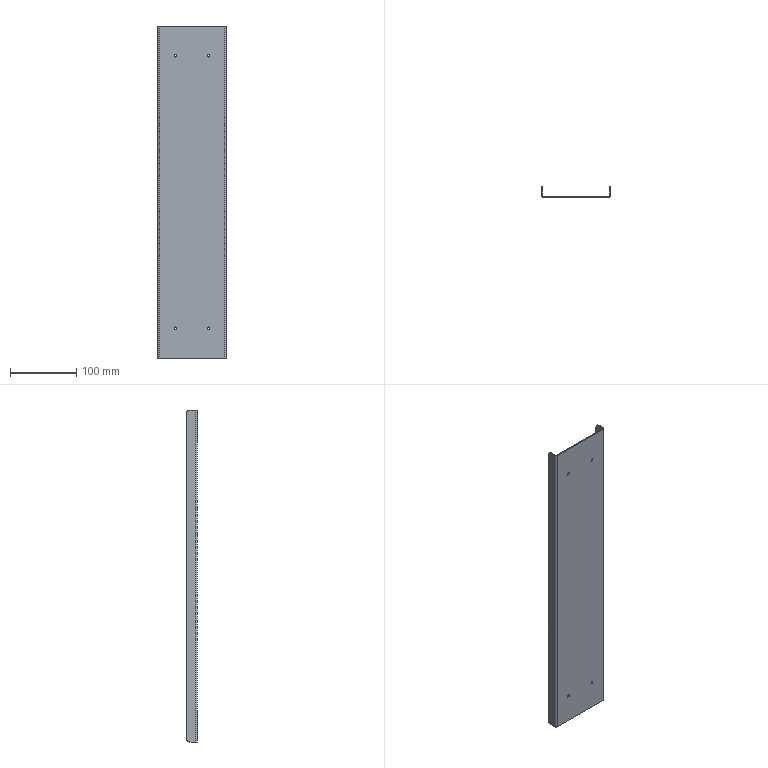Part | SolidWorks | features BreakCorner 1, FlatPattern 1, HoleWzd 1, SMBaseFlange 1, SheetMetal 1 | 1 solid | 34 faces | box 103 x 16.5 x 500 mm | volume 98465 mm3 | plane 18 | cone 8 | cylinder 8 | commonest cylinder face diameters 10 x4 2 x2 5 x2
STEP:
#1=CARTESIAN_POINT('',(25.,-1.5,203.2));
#2=VERTEX_POINT('',#1);
#3=CARTESIAN_POINT('',(25.,-1.5,206.8));
#4=VERTEX_POINT('',#3);
#5=CARTESIAN_POINT('',(25.,-1.5,205.));
#6=DIRECTION('',(0.,1.,0.));
#7=DIRECTION('',(0.,0.,1.));
#8=AXIS2_PLACEMENT_3D('',#5,#6,#7);
#9=CIRCLE('',#8,1.8);
#10=EDGE_CURVE('',#2,#4,#9,.T.);
#11=ORIENTED_EDGE('',*,*,#10,.F.);
#12=CARTESIAN_POINT('',(25.,0.,201.7));
#13=VERTEX_POINT('',#12);
#14=CARTESIAN_POINT('',(25.,0.,201.7));
#15=DIRECTION('',(0.,0.7071,-0.7071));
#16=VECTOR('',#15,1000.);
#17=LINE('',#14,#16);
#18=EDGE_CURVE('',#2,#13,#17,.T.);
#19=ORIENTED_EDGE('',*,*,#18,.T.);
#20=CARTESIAN_POINT('',(25.,0.,208.3));
#21=VERTEX_POINT('',#20);
#22=CARTESIAN_POINT('',(25.,0.,205.));
#23=DIRECTION('',(0.,1.,0.));
#24=DIRECTION('',(0.,0.,1.));
#25=AXIS2_PLACEMENT_3D('',#22,#23,#24);
#26=CIRCLE('',#25,3.3);
#27=EDGE_CURVE('',#13,#21,#26,.T.);
#28=ORIENTED_EDGE('',*,*,#27,.T.);
#29=CARTESIAN_POINT('',(25.,0.,208.3));
#30=DIRECTION('',(0.,0.7071,0.7071));
#31=VECTOR('',#30,1000.);
#32=LINE('',#29,#31);
#33=EDGE_CURVE('',#4,#21,#32,.T.);
#34=ORIENTED_EDGE('',*,*,#33,.F.);
#35=EDGE_LOOP('',(#11,#19,#28,#34));
#36=FACE_OUTER_BOUND('',#35,.T.);
#37=CARTESIAN_POINT('',(25.,0.,205.));
#38=DIRECTION('',(0.,1.,0.));
#39=DIRECTION('',(0.,0.,1.));
#40=AXIS2_PLACEMENT_3D('',#37,#38,#39);
#41=CONICAL_SURFACE('',#40,3.3,0.7854);
#42=ADVANCED_FACE('',(#36),#41,.F.);
#43=CARTESIAN_POINT('',(75.,-1.5,203.2));
#44=VERTEX_POINT('',#43);
#45=CARTESIAN_POINT('',(75.,-1.5,206.8));
#46=VERTEX_POINT('',#45);
#47=CARTESIAN_POINT('',(75.,-1.5,205.));
#48=DIRECTION('',(0.,1.,0.));
#49=DIRECTION('',(0.,0.,1.));
#50=AXIS2_PLACEMENT_3D('',#47,#48,#49);
#51=CIRCLE('',#50,1.8);
#52=EDGE_CURVE('',#44,#46,#51,.T.);
#53=ORIENTED_EDGE('',*,*,#52,.F.);
#54=CARTESIAN_POINT('',(75.,0.,201.7));
#55=VERTEX_POINT('',#54);
#56=CARTESIAN_POINT('',(75.,0.,201.7));
#57=DIRECTION('',(0.,0.7071,-0.7071));
#58=VECTOR('',#57,1000.);
#59=LINE('',#56,#58);
#60=EDGE_CURVE('',#44,#55,#59,.T.);
#61=ORIENTED_EDGE('',*,*,#60,.T.);
#62=CARTESIAN_POINT('',(75.,0.,208.3));
#63=VERTEX_POINT('',#62);
#64=CARTESIAN_POINT('',(75.,0.,205.));
#65=DIRECTION('',(0.,1.,0.));
#66=DIRECTION('',(0.,0.,1.));
#67=AXIS2_PLACEMENT_3D('',#64,#65,#66);
#68=CIRCLE('',#67,3.3);
#69=EDGE_CURVE('',#55,#63,#68,.T.);
#70=ORIENTED_EDGE('',*,*,#69,.T.);
#71=CARTESIAN_POINT('',(75.,0.,208.3));
#72=DIRECTION('',(0.,0.7071,0.7071));
#73=VECTOR('',#72,1000.);
#74=LINE('',#71,#73);
#75=EDGE_CURVE('',#46,#63,#74,.T.);
#76=ORIENTED_EDGE('',*,*,#75,.F.);
#77=EDGE_LOOP('',(#53,#61,#70,#76));
#78=FACE_OUTER_BOUND('',#77,.T.);
#79=CARTESIAN_POINT('',(75.,0.,205.));
#80=DIRECTION('',(0.,1.,0.));
#81=DIRECTION('',(0.,0.,1.));
#82=AXIS2_PLACEMENT_3D('',#79,#80,#81);
#83=CONICAL_SURFACE('',#82,3.3,0.7854);
#84=ADVANCED_FACE('',(#78),#83,.F.);
#85=CARTESIAN_POINT('',(75.,-1.5,-206.8));
#86=VERTEX_POINT('',#85);
#87=CARTESIAN_POINT('',(75.,-1.5,-203.2));
#88=VERTEX_POINT('',#87);
#89=CARTESIAN_POINT('',(75.,-1.5,-205.));
#90=DIRECTION('',(0.,1.,0.));
#91=DIRECTION('',(0.,0.,1.));
#92=AXIS2_PLACEMENT_3D('',#89,#90,#91);
#93=CIRCLE('',#92,1.8);
#94=EDGE_CURVE('',#86,#88,#93,.T.);
#95=ORIENTED_EDGE('',*,*,#94,.F.);
#96=CARTESIAN_POINT('',(75.,0.,-208.3));
#97=VERTEX_POINT('',#96);
#98=CARTESIAN_POINT('',(75.,0.,-208.3));
#99=DIRECTION('',(0.,0.7071,-0.7071));
#100=VECTOR('',#99,1000.);
#101=LINE('',#98,#100);
#102=EDGE_CURVE('',#86,#97,#101,.T.);
#103=ORIENTED_EDGE('',*,*,#102,.T.);
#104=CARTESIAN_POINT('',(75.,0.,-201.7));
#105=VERTEX_POINT('',#104);
#106=CARTESIAN_POINT('',(75.,0.,-205.));
#107=DIRECTION('',(0.,1.,0.));
#108=DIRECTION('',(0.,0.,1.));
#109=AXIS2_PLACEMENT_3D('',#106,#107,#108);
#110=CIRCLE('',#109,3.3);
#111=EDGE_CURVE('',#97,#105,#110,.T.);
#112=ORIENTED_EDGE('',*,*,#111,.T.);
#113=CARTESIAN_POINT('',(75.,0.,-201.7));
#114=DIRECTION('',(0.,0.7071,0.7071));
#115=VECTOR('',#114,1000.);
#116=LINE('',#113,#115);
#117=EDGE_CURVE('',#88,#105,#116,.T.);
#118=ORIENTED_EDGE('',*,*,#117,.F.);
#119=EDGE_LOOP('',(#95,#103,#112,#118));
#120=FACE_OUTER_BOUND('',#119,.T.);
#121=CARTESIAN_POINT('',(75.,0.,-205.));
#122=DIRECTION('',(0.,1.,0.));
#123=DIRECTION('',(0.,0.,1.));
#124=AXIS2_PLACEMENT_3D('',#121,#122,#123);
#125=CONICAL_SURFACE('',#124,3.3,0.7854);
#126=ADVANCED_FACE('',(#120),#125,.F.);
#127=CARTESIAN_POINT('',(25.,-1.5,-206.8));
#128=VERTEX_POINT('',#127);
#129=CARTESIAN_POINT('',(25.,-1.5,-203.2));
#130=VERTEX_POINT('',#129);
#131=CARTESIAN_POINT('',(25.,-1.5,-205.));
#132=DIRECTION('',(0.,1.,0.));
#133=DIRECTION('',(0.,0.,1.));
#134=AXIS2_PLACEMENT_3D('',#131,#132,#133);
#135=CIRCLE('',#134,1.8);
#136=EDGE_CURVE('',#128,#130,#135,.T.);
#137=ORIENTED_EDGE('',*,*,#136,.F.);
#138=CARTESIAN_POINT('',(25.,0.,-208.3));
#139=VERTEX_POINT('',#138);
#140=CARTESIAN_POINT('',(25.,0.,-208.3));
#141=DIRECTION('',(0.,0.7071,-0.7071));
#142=VECTOR('',#141,1000.);
#143=LINE('',#140,#142);
#144=EDGE_CURVE('',#128,#139,#143,.T.);
#145=ORIENTED_EDGE('',*,*,#144,.T.);
#146=CARTESIAN_POINT('',(25.,0.,-201.7));
#147=VERTEX_POINT('',#146);
#148=CARTESIAN_POINT('',(25.,0.,-205.));
#149=DIRECTION('',(0.,1.,0.));
#150=DIRECTION('',(0.,0.,1.));
#151=AXIS2_PLACEMENT_3D('',#148,#149,#150);
#152=CIRCLE('',#151,3.3);
#153=EDGE_CURVE('',#139,#147,#152,.T.);
#154=ORIENTED_EDGE('',*,*,#153,.T.);
#155=CARTESIAN_POINT('',(25.,0.,-201.7));
#156=DIRECTION('',(0.,0.7071,0.7071));
#157=VECTOR('',#156,1000.);
#158=LINE('',#155,#157);
#159=EDGE_CURVE('',#130,#147,#158,.T.);
#160=ORIENTED_EDGE('',*,*,#159,.F.);
#161=EDGE_LOOP('',(#137,#145,#154,#160));
#162=FACE_OUTER_BOUND('',#161,.T.);
#163=CARTESIAN_POINT('',(25.,0.,-205.));
#164=DIRECTION('',(0.,1.,0.));
#165=DIRECTION('',(0.,0.,1.));
#166=AXIS2_PLACEMENT_3D('',#163,#164,#165);
#167=CONICAL_SURFACE('',#166,3.3,0.7854);
#168=ADVANCED_FACE('',(#162),#167,.F.);
#169=CARTESIAN_POINT('',(25.,-1.5,205.));
#170=DIRECTION('',(0.,1.,0.));
#171=DIRECTION('',(0.,0.,1.));
#172=AXIS2_PLACEMENT_3D('',#169,#170,#171);
#173=CIRCLE('',#172,1.8);
#174=EDGE_CURVE('',#4,#2,#173,.T.);
#175=ORIENTED_EDGE('',*,*,#174,.T.);
#176=ORIENTED_EDGE('',*,*,#10,.T.);
#177=EDGE_LOOP('',(#175,#176));
#178=FACE_BOUND('',#177,.T.);
#179=CARTESIAN_POINT('',(75.,-1.5,205.));
#180=DIRECTION('',(0.,1.,0.));
#181=DIRECTION('',(0.,0.,1.));
#182=AXIS2_PLACEMENT_3D('',#179,#180,#181);
#183=CIRCLE('',#182,1.8);
#184=EDGE_CURVE('',#46,#44,#183,.T.);
#185=ORIENTED_EDGE('',*,*,#184,.T.);
#186=ORIENTED_EDGE('',*,*,#52,.T.);
#187=EDGE_LOOP('',(#185,#186));
#188=FACE_BOUND('',#187,.T.);
#189=CARTESIAN_POINT('',(75.,-1.5,-205.));
#190=DIRECTION('',(0.,1.,0.));
#191=DIRECTION('',(0.,0.,1.));
#192=AXIS2_PLACEMENT_3D('',#189,#190,#191);
#193=CIRCLE('',#192,1.8);
#194=EDGE_CURVE('',#88,#86,#193,.T.);
#195=ORIENTED_EDGE('',*,*,#194,.T.);
#196=ORIENTED_EDGE('',*,*,#94,.T.);
#197=EDGE_LOOP('',(#195,#196));
#198=FACE_BOUND('',#197,.T.);
#199=CARTESIAN_POINT('',(25.,-1.5,-205.));
#200=DIRECTION('',(0.,1.,0.));
#201=DIRECTION('',(0.,0.,1.));
#202=AXIS2_PLACEMENT_3D('',#199,#200,#201);
#203=CIRCLE('',#202,1.8);
#204=EDGE_CURVE('',#130,#128,#203,.T.);
#205=ORIENTED_EDGE('',*,*,#204,.T.);
#206=ORIENTED_EDGE('',*,*,#136,.T.);
#207=EDGE_LOOP('',(#205,#206));
#208=FACE_BOUND('',#207,.T.);
#209=CARTESIAN_POINT('',(1.,-1.5,-250.));
#210=VERTEX_POINT('',#209);
#211=CARTESIAN_POINT('',(99.,-1.5,-250.));
#212=VERTEX_POINT('',#211);
#213=CARTESIAN_POINT('',(0.,-1.5,-250.));
#214=DIRECTION('',(1.,0.,0.));
#215=VECTOR('',#214,1000.);
#216=LINE('',#213,#215);
#217=EDGE_CURVE('',#210,#212,#216,.T.);
#218=ORIENTED_EDGE('',*,*,#217,.T.);
#219=CARTESIAN_POINT('',(99.,-1.5,250.));
#220=VERTEX_POINT('',#219);
#221=CARTESIAN_POINT('',(99.,-1.5,250.));
#222=DIRECTION('',(0.,0.,-1.));
#223=VECTOR('',#222,1000.);
#224=LINE('',#221,#223);
#225=EDGE_CURVE('',#220,#212,#224,.T.);
#226=ORIENTED_EDGE('',*,*,#225,.F.);
#227=CARTESIAN_POINT('',(1.,-1.5,250.));
#228=VERTEX_POINT('',#227);
#229=CARTESIAN_POINT('',(0.,-1.5,250.));
#230=DIRECTION('',(1.,0.,0.));
#231=VECTOR('',#230,1000.);
#232=LINE('',#229,#231);
#233=EDGE_CURVE('',#228,#220,#232,.T.);
#234=ORIENTED_EDGE('',*,*,#233,.F.);
#235=CARTESIAN_POINT('',(1.,-1.5,250.));
#236=DIRECTION('',(0.,0.,-1.));
#237=VECTOR('',#236,1000.);
#238=LINE('',#235,#237);
#239=EDGE_CURVE('',#228,#210,#238,.T.);
#240=ORIENTED_EDGE('',*,*,#239,.T.);
#241=EDGE_LOOP('',(#218,#226,#234,#240));
#242=FACE_OUTER_BOUND('',#241,.T.);
#243=CARTESIAN_POINT('',(0.,-1.5,250.));
#244=DIRECTION('',(0.,1.,0.));
#245=DIRECTION('',(0.,0.,1.));
#246=AXIS2_PLACEMENT_3D('',#243,#244,#245);
#247=PLANE('',#246);
#248=ADVANCED_FACE('',(#178,#188,#198,#208,#242),#247,.F.);
#249=CARTESIAN_POINT('',(1.,0.,250.));
#250=VERTEX_POINT('',#249);
#251=CARTESIAN_POINT('',(1.,0.,250.));
#252=DIRECTION('',(0.,-1.,0.));
#253=VECTOR('',#252,1000.);
#254=LINE('',#251,#253);
#255=EDGE_CURVE('',#250,#228,#254,.T.);
#256=ORIENTED_EDGE('',*,*,#255,.F.);
#257=CARTESIAN_POINT('',(0.,1.,250.));
#258=VERTEX_POINT('',#257);
#259=CARTESIAN_POINT('',(1.,1.,250.));
#260=DIRECTION('',(0.,0.,1.));
#261=DIRECTION('',(-1.,0.,0.));
#262=AXIS2_PLACEMENT_3D('',#259,#260,#261);
#263=CIRCLE('',#262,1.);
#264=EDGE_CURVE('',#258,#250,#263,.T.);
#265=ORIENTED_EDGE('',*,*,#264,.F.);
#266=CARTESIAN_POINT('',(-1.5,1.,250.));
#267=VERTEX_POINT('',#266);
#268=CARTESIAN_POINT('',(-1.5,1.,250.));
#269=DIRECTION('',(1.,0.,0.));
#270=VECTOR('',#269,1000.);
#271=LINE('',#268,#270);
#272=EDGE_CURVE('',#267,#258,#271,.T.);
#273=ORIENTED_EDGE('',*,*,#272,.F.);
#274=CARTESIAN_POINT('',(1.,1.,250.));
#275=DIRECTION('',(0.,0.,1.));
#276=DIRECTION('',(1.,0.,0.));
#277=AXIS2_PLACEMENT_3D('',#274,#275,#276);
#278=CIRCLE('',#277,2.5);
#279=EDGE_CURVE('',#267,#228,#278,.T.);
#280=ORIENTED_EDGE('',*,*,#279,.T.);
#281=EDGE_LOOP('',(#256,#265,#273,#280));
#282=FACE_OUTER_BOUND('',#281,.T.);
#283=CARTESIAN_POINT('',(1.,0.,250.));
#284=DIRECTION('',(0.,0.,1.));
#285=DIRECTION('',(1.,0.,0.));
#286=AXIS2_PLACEMENT_3D('',#283,#284,#285);
#287=PLANE('',#286);
#288=ADVANCED_FACE('',(#282),#287,.T.);
#289=CARTESIAN_POINT('',(99.,0.,250.));
#290=VERTEX_POINT('',#289);
#291=CARTESIAN_POINT('',(0.,0.,250.));
#292=DIRECTION('',(1.,0.,0.));
#293=VECTOR('',#292,1000.);
#294=LINE('',#291,#293);
#295=EDGE_CURVE('',#250,#290,#294,.T.);
#296=ORIENTED_EDGE('',*,*,#295,.F.);
#297=ORIENTED_EDGE('',*,*,#255,.T.);
#298=ORIENTED_EDGE('',*,*,#233,.T.);
#299=CARTESIAN_POINT('',(99.,-1.5,250.));
#300=DIRECTION('',(0.,1.,0.));
#301=VECTOR('',#300,1000.);
#302=LINE('',#299,#301);
#303=EDGE_CURVE('',#220,#290,#302,.T.);
#304=ORIENTED_EDGE('',*,*,#303,.T.);
#305=EDGE_LOOP('',(#296,#297,#298,#304));
#306=FACE_OUTER_BOUND('',#305,.T.);
#307=CARTESIAN_POINT('',(-1.5,1.,250.));
#308=DIRECTION('',(0.,0.,1.));
#309=DIRECTION('',(1.,0.,0.));
#310=AXIS2_PLACEMENT_3D('',#307,#308,#309);
#311=PLANE('',#310);
#312=ADVANCED_FACE('',(#306),#311,.T.);
#313=CARTESIAN_POINT('',(0.,1.,-250.));
#314=VERTEX_POINT('',#313);
#315=CARTESIAN_POINT('',(-1.5,1.,-250.));
#316=VERTEX_POINT('',#315);
#317=CARTESIAN_POINT('',(0.,1.,-250.));
#318=DIRECTION('',(-1.,0.,0.));
#319=VECTOR('',#318,1000.);
#320=LINE('',#317,#319);
#321=EDGE_CURVE('',#314,#316,#320,.T.);
#322=ORIENTED_EDGE('',*,*,#321,.F.);
#323=CARTESIAN_POINT('',(1.,0.,-250.));
#324=VERTEX_POINT('',#323);
#325=CARTESIAN_POINT('',(1.,1.,-250.));
#326=DIRECTION('',(0.,0.,1.));
#327=DIRECTION('',(-1.,0.,0.));
#328=AXIS2_PLACEMENT_3D('',#325,#326,#327);
#329=CIRCLE('',#328,1.);
#330=EDGE_CURVE('',#314,#324,#329,.T.);
#331=ORIENTED_EDGE('',*,*,#330,.T.);
#332=CARTESIAN_POINT('',(1.,-1.5,-250.));
#333=DIRECTION('',(0.,1.,0.));
#334=VECTOR('',#333,1000.);
#335=LINE('',#332,#334);
#336=EDGE_CURVE('',#210,#324,#335,.T.);
#337=ORIENTED_EDGE('',*,*,#336,.F.);
#338=CARTESIAN_POINT('',(1.,1.,-250.));
#339=DIRECTION('',(0.,0.,1.));
#340=DIRECTION('',(1.,0.,0.));
#341=AXIS2_PLACEMENT_3D('',#338,#339,#340);
#342=CIRCLE('',#341,2.5);
#343=EDGE_CURVE('',#316,#210,#342,.T.);
#344=ORIENTED_EDGE('',*,*,#343,.F.);
#345=EDGE_LOOP('',(#322,#331,#337,#344));
#346=FACE_OUTER_BOUND('',#345,.T.);
#347=CARTESIAN_POINT('',(0.,1.,-250.));
#348=DIRECTION('',(0.,0.,-1.));
#349=DIRECTION('',(-1.,0.,0.));
#350=AXIS2_PLACEMENT_3D('',#347,#348,#349);
#351=PLANE('',#350);
#352=ADVANCED_FACE('',(#346),#351,.T.);
#353=CARTESIAN_POINT('',(-1.5,10.,-250.));
#354=VERTEX_POINT('',#353);
#355=CARTESIAN_POINT('',(-1.5,15.,-250.));
#356=DIRECTION('',(0.,-1.,0.));
#357=VECTOR('',#356,1000.);
#358=LINE('',#355,#357);
#359=EDGE_CURVE('',#354,#316,#358,.T.);
#360=ORIENTED_EDGE('',*,*,#359,.F.);
#361=CARTESIAN_POINT('',(0.,10.,-250.));
#362=VERTEX_POINT('',#361);
#363=CARTESIAN_POINT('',(1.,10.,-250.));
#364=DIRECTION('',(1.,0.,0.));
#365=VECTOR('',#364,1000.);
#366=LINE('',#363,#365);
#367=EDGE_CURVE('',#354,#362,#366,.T.);
#368=ORIENTED_EDGE('',*,*,#367,.T.);
#369=CARTESIAN_POINT('',(0.,15.,-250.));
#370=DIRECTION('',(0.,-1.,0.));
#371=VECTOR('',#370,1000.);
#372=LINE('',#369,#371);
#373=EDGE_CURVE('',#362,#314,#372,.T.);
#374=ORIENTED_EDGE('',*,*,#373,.T.);
#375=ORIENTED_EDGE('',*,*,#321,.T.);
#376=EDGE_LOOP('',(#360,#368,#374,#375));
#377=FACE_OUTER_BOUND('',#376,.T.);
#378=CARTESIAN_POINT('',(1.,-1.5,-250.));
#379=DIRECTION('',(0.,0.,-1.));
#380=DIRECTION('',(-1.,0.,0.));
#381=AXIS2_PLACEMENT_3D('',#378,#379,#380);
#382=PLANE('',#381);
#383=ADVANCED_FACE('',(#377),#382,.T.);
#384=CARTESIAN_POINT('',(100.,1.,250.));
#385=VERTEX_POINT('',#384);
#386=CARTESIAN_POINT('',(101.5,1.,250.));
#387=VERTEX_POINT('',#386);
#388=CARTESIAN_POINT('',(100.,1.,250.));
#389=DIRECTION('',(1.,0.,0.));
#390=VECTOR('',#389,1000.);
#391=LINE('',#388,#390);
#392=EDGE_CURVE('',#385,#387,#391,.T.);
#393=ORIENTED_EDGE('',*,*,#392,.F.);
#394=CARTESIAN_POINT('',(99.,1.,250.));
#395=DIRECTION('',(0.,0.,1.));
#396=DIRECTION('',(-1.,0.,0.));
#397=AXIS2_PLACEMENT_3D('',#394,#395,#396);
#398=CIRCLE('',#397,1.);
#399=EDGE_CURVE('',#290,#385,#398,.T.);
#400=ORIENTED_EDGE('',*,*,#399,.F.);
#401=ORIENTED_EDGE('',*,*,#303,.F.);
#402=CARTESIAN_POINT('',(99.,1.,250.));
#403=DIRECTION('',(0.,0.,1.));
#404=DIRECTION('',(1.,0.,0.));
#405=AXIS2_PLACEMENT_3D('',#402,#403,#404);
#406=CIRCLE('',#405,2.5);
#407=EDGE_CURVE('',#220,#387,#406,.T.);
#408=ORIENTED_EDGE('',*,*,#407,.T.);
#409=EDGE_LOOP('',(#393,#400,#401,#408));
#410=FACE_OUTER_BOUND('',#409,.T.);
#411=CARTESIAN_POINT('',(100.,1.,250.));
#412=DIRECTION('',(0.,0.,1.));
#413=DIRECTION('',(1.,0.,0.));
#414=AXIS2_PLACEMENT_3D('',#411,#412,#413);
#415=PLANE('',#414);
#416=ADVANCED_FACE('',(#410),#415,.T.);
#417=CARTESIAN_POINT('',(101.5,10.,250.));
#418=VERTEX_POINT('',#417);
#419=CARTESIAN_POINT('',(101.5,0.,250.));
#420=DIRECTION('',(0.,1.,0.));
#421=VECTOR('',#420,1000.);
#422=LINE('',#419,#421);
#423=EDGE_CURVE('',#387,#418,#422,.T.);
#424=ORIENTED_EDGE('',*,*,#423,.T.);
#425=CARTESIAN_POINT('',(100.,10.,250.));
#426=VERTEX_POINT('',#425);
#427=CARTESIAN_POINT('',(99.,10.,250.));
#428=DIRECTION('',(-1.,0.,0.));
#429=VECTOR('',#428,1000.);
#430=LINE('',#427,#429);
#431=EDGE_CURVE('',#418,#426,#430,.T.);
#432=ORIENTED_EDGE('',*,*,#431,.T.);
#433=CARTESIAN_POINT('',(100.,0.,250.));
#434=DIRECTION('',(0.,1.,0.));
#435=VECTOR('',#434,1000.);
#436=LINE('',#433,#435);
#437=EDGE_CURVE('',#385,#426,#436,.T.);
#438=ORIENTED_EDGE('',*,*,#437,.F.);
#439=ORIENTED_EDGE('',*,*,#392,.T.);
#440=EDGE_LOOP('',(#424,#432,#438,#439));
#441=FACE_OUTER_BOUND('',#440,.T.);
#442=CARTESIAN_POINT('',(99.,-1.5,250.));
#443=DIRECTION('',(0.,0.,1.));
#444=DIRECTION('',(1.,0.,0.));
#445=AXIS2_PLACEMENT_3D('',#442,#443,#444);
#446=PLANE('',#445);
#447=ADVANCED_FACE('',(#441),#446,.T.);
#448=CARTESIAN_POINT('',(99.,0.,-250.));
#449=VERTEX_POINT('',#448);
#450=CARTESIAN_POINT('',(99.,0.,-250.));
#451=DIRECTION('',(0.,-1.,0.));
#452=VECTOR('',#451,1000.);
#453=LINE('',#450,#452);
#454=EDGE_CURVE('',#449,#212,#453,.T.);
#455=ORIENTED_EDGE('',*,*,#454,.F.);
#456=CARTESIAN_POINT('',(100.,1.,-250.));
#457=VERTEX_POINT('',#456);
#458=CARTESIAN_POINT('',(99.,1.,-250.));
#459=DIRECTION('',(0.,0.,1.));
#460=DIRECTION('',(-1.,0.,0.));
#461=AXIS2_PLACEMENT_3D('',#458,#459,#460);
#462=CIRCLE('',#461,1.);
#463=EDGE_CURVE('',#449,#457,#462,.T.);
#464=ORIENTED_EDGE('',*,*,#463,.T.);
#465=CARTESIAN_POINT('',(101.5,1.,-250.));
#466=VERTEX_POINT('',#465);
#467=CARTESIAN_POINT('',(101.5,1.,-250.));
#468=DIRECTION('',(-1.,0.,0.));
#469=VECTOR('',#468,1000.);
#470=LINE('',#467,#469);
#471=EDGE_CURVE('',#466,#457,#470,.T.);
#472=ORIENTED_EDGE('',*,*,#471,.F.);
#473=CARTESIAN_POINT('',(99.,1.,-250.));
#474=DIRECTION('',(0.,0.,1.));
#475=DIRECTION('',(1.,0.,0.));
#476=AXIS2_PLACEMENT_3D('',#473,#474,#475);
#477=CIRCLE('',#476,2.5);
#478=EDGE_CURVE('',#212,#466,#477,.T.);
#479=ORIENTED_EDGE('',*,*,#478,.F.);
#480=EDGE_LOOP('',(#455,#464,#472,#479));
#481=FACE_OUTER_BOUND('',#480,.T.);
#482=CARTESIAN_POINT('',(99.,0.,-250.));
#483=DIRECTION('',(0.,0.,-1.));
#484=DIRECTION('',(-1.,0.,0.));
#485=AXIS2_PLACEMENT_3D('',#482,#483,#484);
#486=PLANE('',#485);
#487=ADVANCED_FACE('',(#481),#486,.T.);
#488=CARTESIAN_POINT('',(0.,0.,-250.));
#489=DIRECTION('',(1.,0.,0.));
#490=VECTOR('',#489,1000.);
#491=LINE('',#488,#490);
#492=EDGE_CURVE('',#324,#449,#491,.T.);
#493=ORIENTED_EDGE('',*,*,#492,.T.);
#494=ORIENTED_EDGE('',*,*,#454,.T.);
#495=ORIENTED_EDGE('',*,*,#217,.F.);
#496=ORIENTED_EDGE('',*,*,#336,.T.);
#497=EDGE_LOOP('',(#493,#494,#495,#496));
#498=FACE_OUTER_BOUND('',#497,.T.);
#499=CARTESIAN_POINT('',(101.5,1.,-250.));
#500=DIRECTION('',(0.,0.,-1.));
#501=DIRECTION('',(-1.,0.,0.));
#502=AXIS2_PLACEMENT_3D('',#499,#500,#501);
#503=PLANE('',#502);
#504=ADVANCED_FACE('',(#498),#503,.T.);
#505=CARTESIAN_POINT('',(101.5,15.,245.));
#506=VERTEX_POINT('',#505);
#507=CARTESIAN_POINT('',(101.5,15.,-245.));
#508=VERTEX_POINT('',#507);
#509=CARTESIAN_POINT('',(101.5,15.,250.));
#510=DIRECTION('',(0.,0.,-1.));
#511=VECTOR('',#510,1000.);
#512=LINE('',#509,#511);
#513=EDGE_CURVE('',#506,#508,#512,.T.);
#514=ORIENTED_EDGE('',*,*,#513,.F.);
#515=CARTESIAN_POINT('',(101.5,10.,245.));
#516=DIRECTION('',(1.,0.,0.));
#517=DIRECTION('',(0.,0.,1.));
#518=AXIS2_PLACEMENT_3D('',#515,#516,#517);
#519=CIRCLE('',#518,5.);
#520=EDGE_CURVE('',#506,#418,#519,.T.);
#521=ORIENTED_EDGE('',*,*,#520,.T.);
#522=ORIENTED_EDGE('',*,*,#423,.F.);
#523=CARTESIAN_POINT('',(101.5,1.,250.));
#524=DIRECTION('',(0.,0.,-1.));
#525=VECTOR('',#524,1000.);
#526=LINE('',#523,#525);
#527=EDGE_CURVE('',#387,#466,#526,.T.);
#528=ORIENTED_EDGE('',*,*,#527,.T.);
#529=CARTESIAN_POINT('',(101.5,10.,-250.));
#530=VERTEX_POINT('',#529);
#531=CARTESIAN_POINT('',(101.5,0.,-250.));
#532=DIRECTION('',(0.,1.,0.));
#533=VECTOR('',#532,1000.);
#534=LINE('',#531,#533);
#535=EDGE_CURVE('',#466,#530,#534,.T.);
#536=ORIENTED_EDGE('',*,*,#535,.T.);
#537=CARTESIAN_POINT('',(101.5,10.,-245.));
#538=DIRECTION('',(1.,0.,0.));
#539=DIRECTION('',(0.,0.,1.));
#540=AXIS2_PLACEMENT_3D('',#537,#538,#539);
#541=CIRCLE('',#540,5.);
#542=EDGE_CURVE('',#530,#508,#541,.T.);
#543=ORIENTED_EDGE('',*,*,#542,.T.);
#544=EDGE_LOOP('',(#514,#521,#522,#528,#536,#543));
#545=FACE_OUTER_BOUND('',#544,.T.);
#546=CARTESIAN_POINT('',(101.5,0.,250.));
#547=DIRECTION('',(-1.,0.,0.));
#548=DIRECTION('',(0.,0.,1.));
#549=AXIS2_PLACEMENT_3D('',#546,#547,#548);
#550=PLANE('',#549);
#551=ADVANCED_FACE('',(#545),#550,.F.);
#552=CARTESIAN_POINT('',(100.,15.,245.));
#553=VERTEX_POINT('',#552);
#554=CARTESIAN_POINT('',(100.,15.,-245.));
#555=VERTEX_POINT('',#554);
#556=CARTESIAN_POINT('',(100.,15.,250.));
#557=DIRECTION('',(0.,0.,-1.));
#558=VECTOR('',#557,1000.);
#559=LINE('',#556,#558);
#560=EDGE_CURVE('',#553,#555,#559,.T.);
#561=ORIENTED_EDGE('',*,*,#560,.F.);
#562=CARTESIAN_POINT('',(100.,15.,245.));
#563=DIRECTION('',(1.,0.,0.));
#564=VECTOR('',#563,1000.);
#565=LINE('',#562,#564);
#566=EDGE_CURVE('',#553,#506,#565,.T.);
#567=ORIENTED_EDGE('',*,*,#566,.T.);
#568=ORIENTED_EDGE('',*,*,#513,.T.);
#569=CARTESIAN_POINT('',(100.,15.,-245.));
#570=DIRECTION('',(-1.,0.,0.));
#571=VECTOR('',#570,1000.);
#572=LINE('',#569,#571);
#573=EDGE_CURVE('',#508,#555,#572,.T.);
#574=ORIENTED_EDGE('',*,*,#573,.T.);
#575=EDGE_LOOP('',(#561,#567,#568,#574));
#576=FACE_OUTER_BOUND('',#575,.T.);
#577=CARTESIAN_POINT('',(100.,15.,250.));
#578=DIRECTION('',(0.,1.,0.));
#579=DIRECTION('',(0.,0.,1.));
#580=AXIS2_PLACEMENT_3D('',#577,#578,#579);
#581=PLANE('',#580);
#582=ADVANCED_FACE('',(#576),#581,.T.);
#583=ORIENTED_EDGE('',*,*,#437,.T.);
#584=CARTESIAN_POINT('',(100.,10.,245.));
#585=DIRECTION('',(-1.,0.,0.));
#586=DIRECTION('',(0.,0.,1.));
#587=AXIS2_PLACEMENT_3D('',#584,#585,#586);
#588=CIRCLE('',#587,5.);
#589=EDGE_CURVE('',#426,#553,#588,.T.);
#590=ORIENTED_EDGE('',*,*,#589,.T.);
#591=ORIENTED_EDGE('',*,*,#560,.T.);
#592=CARTESIAN_POINT('',(100.,10.,-250.));
#593=VERTEX_POINT('',#592);
#594=CARTESIAN_POINT('',(100.,10.,-245.));
#595=DIRECTION('',(-1.,0.,0.));
#596=DIRECTION('',(0.,0.,1.));
#597=AXIS2_PLACEMENT_3D('',#594,#595,#596);
#598=CIRCLE('',#597,5.);
#599=EDGE_CURVE('',#555,#593,#598,.T.);
#600=ORIENTED_EDGE('',*,*,#599,.T.);
#601=CARTESIAN_POINT('',(100.,0.,-250.));
#602=DIRECTION('',(0.,1.,0.));
#603=VECTOR('',#602,1000.);
#604=LINE('',#601,#603);
#605=EDGE_CURVE('',#457,#593,#604,.T.);
#606=ORIENTED_EDGE('',*,*,#605,.F.);
#607=CARTESIAN_POINT('',(100.,1.,250.));
#608=DIRECTION('',(0.,0.,-1.));
#609=VECTOR('',#608,1000.);
#610=LINE('',#607,#609);
#611=EDGE_CURVE('',#385,#457,#610,.T.);
#612=ORIENTED_EDGE('',*,*,#611,.F.);
#613=EDGE_LOOP('',(#583,#590,#591,#600,#606,#612));
#614=FACE_OUTER_BOUND('',#613,.T.);
#615=CARTESIAN_POINT('',(100.,0.,250.));
#616=DIRECTION('',(-1.,0.,0.));
#617=DIRECTION('',(0.,0.,1.));
#618=AXIS2_PLACEMENT_3D('',#615,#616,#617);
#619=PLANE('',#618);
#620=ADVANCED_FACE('',(#614),#619,.T.);
#621=ORIENTED_EDGE('',*,*,#463,.F.);
#622=CARTESIAN_POINT('',(99.,0.,250.));
#623=DIRECTION('',(0.,0.,-1.));
#624=VECTOR('',#623,1000.);
#625=LINE('',#622,#624);
#626=EDGE_CURVE('',#290,#449,#625,.T.);
#627=ORIENTED_EDGE('',*,*,#626,.F.);
#628=ORIENTED_EDGE('',*,*,#399,.T.);
#629=ORIENTED_EDGE('',*,*,#611,.T.);
#630=EDGE_LOOP('',(#621,#627,#628,#629));
#631=FACE_OUTER_BOUND('',#630,.T.);
#632=CARTESIAN_POINT('',(99.,1.,250.));
#633=DIRECTION('',(0.,0.,-1.));
#634=DIRECTION('',(-1.,0.,0.));
#635=AXIS2_PLACEMENT_3D('',#632,#633,#634);
#636=CYLINDRICAL_SURFACE('',#635,1.);
#637=ADVANCED_FACE('',(#631),#636,.F.);
#638=CARTESIAN_POINT('',(25.,0.,205.));
#639=DIRECTION('',(0.,1.,0.));
#640=DIRECTION('',(0.,0.,1.));
#641=AXIS2_PLACEMENT_3D('',#638,#639,#640);
#642=CIRCLE('',#641,3.3);
#643=EDGE_CURVE('',#21,#13,#642,.T.);
#644=ORIENTED_EDGE('',*,*,#643,.F.);
#645=ORIENTED_EDGE('',*,*,#27,.F.);
#646=EDGE_LOOP('',(#644,#645));
#647=FACE_BOUND('',#646,.T.);
#648=CARTESIAN_POINT('',(75.,0.,205.));
#649=DIRECTION('',(0.,1.,0.));
#650=DIRECTION('',(0.,0.,1.));
#651=AXIS2_PLACEMENT_3D('',#648,#649,#650);
#652=CIRCLE('',#651,3.3);
#653=EDGE_CURVE('',#63,#55,#652,.T.);
#654=ORIENTED_EDGE('',*,*,#653,.F.);
#655=ORIENTED_EDGE('',*,*,#69,.F.);
#656=EDGE_LOOP('',(#654,#655));
#657=FACE_BOUND('',#656,.T.);
#658=CARTESIAN_POINT('',(75.,0.,-205.));
#659=DIRECTION('',(0.,1.,0.));
#660=DIRECTION('',(0.,0.,1.));
#661=AXIS2_PLACEMENT_3D('',#658,#659,#660);
#662=CIRCLE('',#661,3.3);
#663=EDGE_CURVE('',#105,#97,#662,.T.);
#664=ORIENTED_EDGE('',*,*,#663,.F.);
#665=ORIENTED_EDGE('',*,*,#111,.F.);
#666=EDGE_LOOP('',(#664,#665));
#667=FACE_BOUND('',#666,.T.);
#668=CARTESIAN_POINT('',(25.,0.,-205.));
#669=DIRECTION('',(0.,1.,0.));
#670=DIRECTION('',(0.,0.,1.));
#671=AXIS2_PLACEMENT_3D('',#668,#669,#670);
#672=CIRCLE('',#671,3.3);
#673=EDGE_CURVE('',#147,#139,#672,.T.);
#674=ORIENTED_EDGE('',*,*,#673,.F.);
#675=ORIENTED_EDGE('',*,*,#153,.F.);
#676=EDGE_LOOP('',(#674,#675));
#677=FACE_BOUND('',#676,.T.);
#678=ORIENTED_EDGE('',*,*,#492,.F.);
#679=CARTESIAN_POINT('',(1.,0.,250.));
#680=DIRECTION('',(0.,0.,-1.));
#681=VECTOR('',#680,1000.);
#682=LINE('',#679,#681);
#683=EDGE_CURVE('',#250,#324,#682,.T.);
#684=ORIENTED_EDGE('',*,*,#683,.F.);
#685=ORIENTED_EDGE('',*,*,#295,.T.);
#686=ORIENTED_EDGE('',*,*,#626,.T.);
#687=EDGE_LOOP('',(#678,#684,#685,#686));
#688=FACE_OUTER_BOUND('',#687,.T.);
#689=CARTESIAN_POINT('',(0.,0.,250.));
#690=DIRECTION('',(0.,1.,0.));
#691=DIRECTION('',(0.,0.,1.));
#692=AXIS2_PLACEMENT_3D('',#689,#690,#691);
#693=PLANE('',#692);
#694=ADVANCED_FACE('',(#647,#657,#667,#677,#688),#693,.T.);
#695=ORIENTED_EDGE('',*,*,#330,.F.);
#696=CARTESIAN_POINT('',(0.,1.,250.));
#697=DIRECTION('',(0.,0.,-1.));
#698=VECTOR('',#697,1000.);
#699=LINE('',#696,#698);
#700=EDGE_CURVE('',#258,#314,#699,.T.);
#701=ORIENTED_EDGE('',*,*,#700,.F.);
#702=ORIENTED_EDGE('',*,*,#264,.T.);
#703=ORIENTED_EDGE('',*,*,#683,.T.);
#704=EDGE_LOOP('',(#695,#701,#702,#703));
#705=FACE_OUTER_BOUND('',#704,.T.);
#706=CARTESIAN_POINT('',(1.,1.,250.));
#707=DIRECTION('',(0.,0.,-1.));
#708=DIRECTION('',(-1.,0.,0.));
#709=AXIS2_PLACEMENT_3D('',#706,#707,#708);
#710=CYLINDRICAL_SURFACE('',#709,1.);
#711=ADVANCED_FACE('',(#705),#710,.F.);
#712=CARTESIAN_POINT('',(0.,15.,245.));
#713=VERTEX_POINT('',#712);
#714=CARTESIAN_POINT('',(0.,15.,-245.));
#715=VERTEX_POINT('',#714);
#716=CARTESIAN_POINT('',(0.,15.,250.));
#717=DIRECTION('',(0.,0.,-1.));
#718=VECTOR('',#717,1000.);
#719=LINE('',#716,#718);
#720=EDGE_CURVE('',#713,#715,#719,.T.);
#721=ORIENTED_EDGE('',*,*,#720,.F.);
#722=CARTESIAN_POINT('',(0.,10.,250.));
#723=VERTEX_POINT('',#722);
#724=CARTESIAN_POINT('',(0.,10.,245.));
#725=DIRECTION('',(1.,0.,0.));
#726=DIRECTION('',(0.,1.,0.));
#727=AXIS2_PLACEMENT_3D('',#724,#725,#726);
#728=CIRCLE('',#727,5.);
#729=EDGE_CURVE('',#713,#723,#728,.T.);
#730=ORIENTED_EDGE('',*,*,#729,.T.);
#731=CARTESIAN_POINT('',(0.,15.,250.));
#732=DIRECTION('',(0.,-1.,0.));
#733=VECTOR('',#732,1000.);
#734=LINE('',#731,#733);
#735=EDGE_CURVE('',#723,#258,#734,.T.);
#736=ORIENTED_EDGE('',*,*,#735,.T.);
#737=ORIENTED_EDGE('',*,*,#700,.T.);
#738=ORIENTED_EDGE('',*,*,#373,.F.);
#739=CARTESIAN_POINT('',(0.,10.,-245.));
#740=DIRECTION('',(1.,0.,0.));
#741=DIRECTION('',(0.,1.,0.));
#742=AXIS2_PLACEMENT_3D('',#739,#740,#741);
#743=CIRCLE('',#742,5.);
#744=EDGE_CURVE('',#362,#715,#743,.T.);
#745=ORIENTED_EDGE('',*,*,#744,.T.);
#746=EDGE_LOOP('',(#721,#730,#736,#737,#738,#745));
#747=FACE_OUTER_BOUND('',#746,.T.);
#748=CARTESIAN_POINT('',(0.,15.,250.));
#749=DIRECTION('',(1.,0.,0.));
#750=DIRECTION('',(0.,1.,0.));
#751=AXIS2_PLACEMENT_3D('',#748,#749,#750);
#752=PLANE('',#751);
#753=ADVANCED_FACE('',(#747),#752,.T.);
#754=CARTESIAN_POINT('',(-1.5,15.,245.));
#755=VERTEX_POINT('',#754);
#756=CARTESIAN_POINT('',(-1.5,15.,-245.));
#757=VERTEX_POINT('',#756);
#758=CARTESIAN_POINT('',(-1.5,15.,250.));
#759=DIRECTION('',(0.,0.,-1.));
#760=VECTOR('',#759,1000.);
#761=LINE('',#758,#760);
#762=EDGE_CURVE('',#755,#757,#761,.T.);
#763=ORIENTED_EDGE('',*,*,#762,.F.);
#764=CARTESIAN_POINT('',(0.,15.,245.));
#765=DIRECTION('',(1.,0.,0.));
#766=VECTOR('',#765,1000.);
#767=LINE('',#764,#766);
#768=EDGE_CURVE('',#755,#713,#767,.T.);
#769=ORIENTED_EDGE('',*,*,#768,.T.);
#770=ORIENTED_EDGE('',*,*,#720,.T.);
#771=CARTESIAN_POINT('',(-1.5,15.,-245.));
#772=DIRECTION('',(-1.,0.,0.));
#773=VECTOR('',#772,1000.);
#774=LINE('',#771,#773);
#775=EDGE_CURVE('',#715,#757,#774,.T.);
#776=ORIENTED_EDGE('',*,*,#775,.T.);
#777=EDGE_LOOP('',(#763,#769,#770,#776));
#778=FACE_OUTER_BOUND('',#777,.T.);
#779=CARTESIAN_POINT('',(-1.5,15.,250.));
#780=DIRECTION('',(0.,1.,0.));
#781=DIRECTION('',(-1.,0.,0.));
#782=AXIS2_PLACEMENT_3D('',#779,#780,#781);
#783=PLANE('',#782);
#784=ADVANCED_FACE('',(#778),#783,.T.);
#785=CARTESIAN_POINT('',(-1.5,10.,250.));
#786=VERTEX_POINT('',#785);
#787=CARTESIAN_POINT('',(-1.5,15.,250.));
#788=DIRECTION('',(0.,-1.,0.));
#789=VECTOR('',#788,1000.);
#790=LINE('',#787,#789);
#791=EDGE_CURVE('',#786,#267,#790,.T.);
#792=ORIENTED_EDGE('',*,*,#791,.F.);
#793=CARTESIAN_POINT('',(-1.5,10.,245.));
#794=DIRECTION('',(-1.,0.,0.));
#795=DIRECTION('',(0.,1.,0.));
#796=AXIS2_PLACEMENT_3D('',#793,#794,#795);
#797=CIRCLE('',#796,5.);
#798=EDGE_CURVE('',#786,#755,#797,.T.);
#799=ORIENTED_EDGE('',*,*,#798,.T.);
#800=ORIENTED_EDGE('',*,*,#762,.T.);
#801=CARTESIAN_POINT('',(-1.5,10.,-245.));
#802=DIRECTION('',(-1.,0.,0.));
#803=DIRECTION('',(0.,1.,0.));
#804=AXIS2_PLACEMENT_3D('',#801,#802,#803);
#805=CIRCLE('',#804,5.);
#806=EDGE_CURVE('',#757,#354,#805,.T.);
#807=ORIENTED_EDGE('',*,*,#806,.T.);
#808=ORIENTED_EDGE('',*,*,#359,.T.);
#809=CARTESIAN_POINT('',(-1.5,1.,250.));
#810=DIRECTION('',(0.,0.,-1.));
#811=VECTOR('',#810,1000.);
#812=LINE('',#809,#811);
#813=EDGE_CURVE('',#267,#316,#812,.T.);
#814=ORIENTED_EDGE('',*,*,#813,.F.);
#815=EDGE_LOOP('',(#792,#799,#800,#807,#808,#814));
#816=FACE_OUTER_BOUND('',#815,.T.);
#817=CARTESIAN_POINT('',(-1.5,15.,250.));
#818=DIRECTION('',(1.,0.,0.));
#819=DIRECTION('',(0.,1.,0.));
#820=AXIS2_PLACEMENT_3D('',#817,#818,#819);
#821=PLANE('',#820);
#822=ADVANCED_FACE('',(#816),#821,.F.);
#823=ORIENTED_EDGE('',*,*,#343,.T.);
#824=ORIENTED_EDGE('',*,*,#239,.F.);
#825=ORIENTED_EDGE('',*,*,#279,.F.);
#826=ORIENTED_EDGE('',*,*,#813,.T.);
#827=EDGE_LOOP('',(#823,#824,#825,#826));
#828=FACE_OUTER_BOUND('',#827,.T.);
#829=CARTESIAN_POINT('',(1.,1.,250.));
#830=DIRECTION('',(0.,0.,-1.));
#831=DIRECTION('',(-1.,0.,0.));
#832=AXIS2_PLACEMENT_3D('',#829,#830,#831);
#833=CYLINDRICAL_SURFACE('',#832,2.5);
#834=ADVANCED_FACE('',(#828),#833,.T.);
#835=ORIENTED_EDGE('',*,*,#478,.T.);
#836=ORIENTED_EDGE('',*,*,#527,.F.);
#837=ORIENTED_EDGE('',*,*,#407,.F.);
#838=ORIENTED_EDGE('',*,*,#225,.T.);
#839=EDGE_LOOP('',(#835,#836,#837,#838));
#840=FACE_OUTER_BOUND('',#839,.T.);
#841=CARTESIAN_POINT('',(99.,1.,250.));
#842=DIRECTION('',(0.,0.,-1.));
#843=DIRECTION('',(-1.,0.,0.));
#844=AXIS2_PLACEMENT_3D('',#841,#842,#843);
#845=CYLINDRICAL_SURFACE('',#844,2.5);
#846=ADVANCED_FACE('',(#840),#845,.T.);
#847=ORIENTED_EDGE('',*,*,#735,.F.);
#848=CARTESIAN_POINT('',(-1.5,10.,250.));
#849=DIRECTION('',(-1.,0.,0.));
#850=VECTOR('',#849,1000.);
#851=LINE('',#848,#850);
#852=EDGE_CURVE('',#723,#786,#851,.T.);
#853=ORIENTED_EDGE('',*,*,#852,.T.);
#854=ORIENTED_EDGE('',*,*,#791,.T.);
#855=ORIENTED_EDGE('',*,*,#272,.T.);
#856=EDGE_LOOP('',(#847,#853,#854,#855));
#857=FACE_OUTER_BOUND('',#856,.T.);
#858=CARTESIAN_POINT('',(99.,1.,250.));
#859=DIRECTION('',(0.,0.,-1.));
#860=DIRECTION('',(-1.,0.,0.));
#861=AXIS2_PLACEMENT_3D('',#858,#859,#860);
#862=PLANE('',#861);
#863=ADVANCED_FACE('',(#857),#862,.F.);
#864=ORIENTED_EDGE('',*,*,#605,.T.);
#865=CARTESIAN_POINT('',(99.,10.,-250.));
#866=DIRECTION('',(1.,0.,0.));
#867=VECTOR('',#866,1000.);
#868=LINE('',#865,#867);
#869=EDGE_CURVE('',#593,#530,#868,.T.);
#870=ORIENTED_EDGE('',*,*,#869,.T.);
#871=ORIENTED_EDGE('',*,*,#535,.F.);
#872=ORIENTED_EDGE('',*,*,#471,.T.);
#873=EDGE_LOOP('',(#864,#870,#871,#872));
#874=FACE_OUTER_BOUND('',#873,.T.);
#875=CARTESIAN_POINT('',(99.,1.,-250.));
#876=DIRECTION('',(0.,0.,-1.));
#877=DIRECTION('',(-1.,0.,0.));
#878=AXIS2_PLACEMENT_3D('',#875,#876,#877);
#879=PLANE('',#878);
#880=ADVANCED_FACE('',(#874),#879,.T.);
#881=ORIENTED_EDGE('',*,*,#798,.F.);
#882=ORIENTED_EDGE('',*,*,#852,.F.);
#883=ORIENTED_EDGE('',*,*,#729,.F.);
#884=ORIENTED_EDGE('',*,*,#768,.F.);
#885=EDGE_LOOP('',(#881,#882,#883,#884));
#886=FACE_OUTER_BOUND('',#885,.T.);
#887=CARTESIAN_POINT('',(-1.5,10.,245.));
#888=DIRECTION('',(-1.,0.,0.));
#889=DIRECTION('',(0.,-1.,0.));
#890=AXIS2_PLACEMENT_3D('',#887,#888,#889);
#891=CYLINDRICAL_SURFACE('',#890,5.);
#892=ADVANCED_FACE('',(#886),#891,.T.);
#893=ORIENTED_EDGE('',*,*,#806,.F.);
#894=ORIENTED_EDGE('',*,*,#775,.F.);
#895=ORIENTED_EDGE('',*,*,#744,.F.);
#896=ORIENTED_EDGE('',*,*,#367,.F.);
#897=EDGE_LOOP('',(#893,#894,#895,#896));
#898=FACE_OUTER_BOUND('',#897,.T.);
#899=CARTESIAN_POINT('',(1.,10.,-245.));
#900=DIRECTION('',(1.,0.,0.));
#901=DIRECTION('',(0.,1.,0.));
#902=AXIS2_PLACEMENT_3D('',#899,#900,#901);
#903=CYLINDRICAL_SURFACE('',#902,5.);
#904=ADVANCED_FACE('',(#898),#903,.T.);
#905=ORIENTED_EDGE('',*,*,#589,.F.);
#906=ORIENTED_EDGE('',*,*,#431,.F.);
#907=ORIENTED_EDGE('',*,*,#520,.F.);
#908=ORIENTED_EDGE('',*,*,#566,.F.);
#909=EDGE_LOOP('',(#905,#906,#907,#908));
#910=FACE_OUTER_BOUND('',#909,.T.);
#911=CARTESIAN_POINT('',(100.,10.,245.));
#912=DIRECTION('',(1.,0.,0.));
#913=DIRECTION('',(0.,0.,-1.));
#914=AXIS2_PLACEMENT_3D('',#911,#912,#913);
#915=CYLINDRICAL_SURFACE('',#914,5.);
#916=ADVANCED_FACE('',(#910),#915,.T.);
#917=ORIENTED_EDGE('',*,*,#599,.F.);
#918=ORIENTED_EDGE('',*,*,#573,.F.);
#919=ORIENTED_EDGE('',*,*,#542,.F.);
#920=ORIENTED_EDGE('',*,*,#869,.F.);
#921=EDGE_LOOP('',(#917,#918,#919,#920));
#922=FACE_OUTER_BOUND('',#921,.T.);
#923=CARTESIAN_POINT('',(99.,10.,-245.));
#924=DIRECTION('',(1.,0.,0.));
#925=DIRECTION('',(0.,0.,-1.));
#926=AXIS2_PLACEMENT_3D('',#923,#924,#925);
#927=CYLINDRICAL_SURFACE('',#926,5.);
#928=ADVANCED_FACE('',(#922),#927,.T.);
#929=ORIENTED_EDGE('',*,*,#144,.F.);
#930=ORIENTED_EDGE('',*,*,#204,.F.);
#931=ORIENTED_EDGE('',*,*,#159,.T.);
#932=ORIENTED_EDGE('',*,*,#673,.T.);
#933=EDGE_LOOP('',(#929,#930,#931,#932));
#934=FACE_OUTER_BOUND('',#933,.T.);
#935=CARTESIAN_POINT('',(25.,0.,-205.));
#936=DIRECTION('',(0.,1.,0.));
#937=DIRECTION('',(0.,0.,1.));
#938=AXIS2_PLACEMENT_3D('',#935,#936,#937);
#939=CONICAL_SURFACE('',#938,3.3,0.7854);
#940=ADVANCED_FACE('',(#934),#939,.F.);
#941=ORIENTED_EDGE('',*,*,#102,.F.);
#942=ORIENTED_EDGE('',*,*,#194,.F.);
#943=ORIENTED_EDGE('',*,*,#117,.T.);
#944=ORIENTED_EDGE('',*,*,#663,.T.);
#945=EDGE_LOOP('',(#941,#942,#943,#944));
#946=FACE_OUTER_BOUND('',#945,.T.);
#947=CARTESIAN_POINT('',(75.,0.,-205.));
#948=DIRECTION('',(0.,1.,0.));
#949=DIRECTION('',(0.,0.,1.));
#950=AXIS2_PLACEMENT_3D('',#947,#948,#949);
#951=CONICAL_SURFACE('',#950,3.3,0.7854);
#952=ADVANCED_FACE('',(#946),#951,.F.);
#953=ORIENTED_EDGE('',*,*,#60,.F.);
#954=ORIENTED_EDGE('',*,*,#184,.F.);
#955=ORIENTED_EDGE('',*,*,#75,.T.);
#956=ORIENTED_EDGE('',*,*,#653,.T.);
#957=EDGE_LOOP('',(#953,#954,#955,#956));
#958=FACE_OUTER_BOUND('',#957,.T.);
#959=CARTESIAN_POINT('',(75.,0.,205.));
#960=DIRECTION('',(0.,1.,0.));
#961=DIRECTION('',(0.,0.,1.));
#962=AXIS2_PLACEMENT_3D('',#959,#960,#961);
#963=CONICAL_SURFACE('',#962,3.3,0.7854);
#964=ADVANCED_FACE('',(#958),#963,.F.);
#965=ORIENTED_EDGE('',*,*,#18,.F.);
#966=ORIENTED_EDGE('',*,*,#174,.F.);
#967=ORIENTED_EDGE('',*,*,#33,.T.);
#968=ORIENTED_EDGE('',*,*,#643,.T.);
#969=EDGE_LOOP('',(#965,#966,#967,#968));
#970=FACE_OUTER_BOUND('',#969,.T.);
#971=CARTESIAN_POINT('',(25.,0.,205.));
#972=DIRECTION('',(0.,1.,0.));
#973=DIRECTION('',(0.,0.,1.));
#974=AXIS2_PLACEMENT_3D('',#971,#972,#973);
#975=CONICAL_SURFACE('',#974,3.3,0.7854);
#976=ADVANCED_FACE('',(#970),#975,.F.);
#977=CLOSED_SHELL('',(#42,#84,#126,#168,#248,#288,#312,#352,#383,#416,#447,#487,#504,#551,#582,#620,#637,#694,#711,#753,#784,#822,#834,#846,#863,#880,#892,#904,#916,#928,#940,#952,#964,#976));
#978=MANIFOLD_SOLID_BREP('',#977);
#979=CARTESIAN_POINT('',(0.,0.,0.));
#980=DIRECTION('',(0.,0.,1.));
#981=DIRECTION('',(1.,0.,0.));
#982=AXIS2_PLACEMENT_3D('',#979,#980,#981);
#983=(LENGTH_UNIT()NAMED_UNIT(*)SI_UNIT(.MILLI.,.METRE.));
#984=UNCERTAINTY_MEASURE_WITH_UNIT(LENGTH_MEASURE(0.00001),#983,'','');
#985=(NAMED_UNIT(*)PLANE_ANGLE_UNIT()SI_UNIT($,.RADIAN.));
#986=(NAMED_UNIT(*)SI_UNIT($,.STERADIAN.)SOLID_ANGLE_UNIT());
#987=(GEOMETRIC_REPRESENTATION_CONTEXT(3)GLOBAL_UNCERTAINTY_ASSIGNED_CONTEXT((#984))GLOBAL_UNIT_ASSIGNED_CONTEXT((#983,#985,#986))REPRESENTATION_CONTEXT('',''));
#988=ADVANCED_BREP_SHAPE_REPRESENTATION('',(#978,#982),#987);